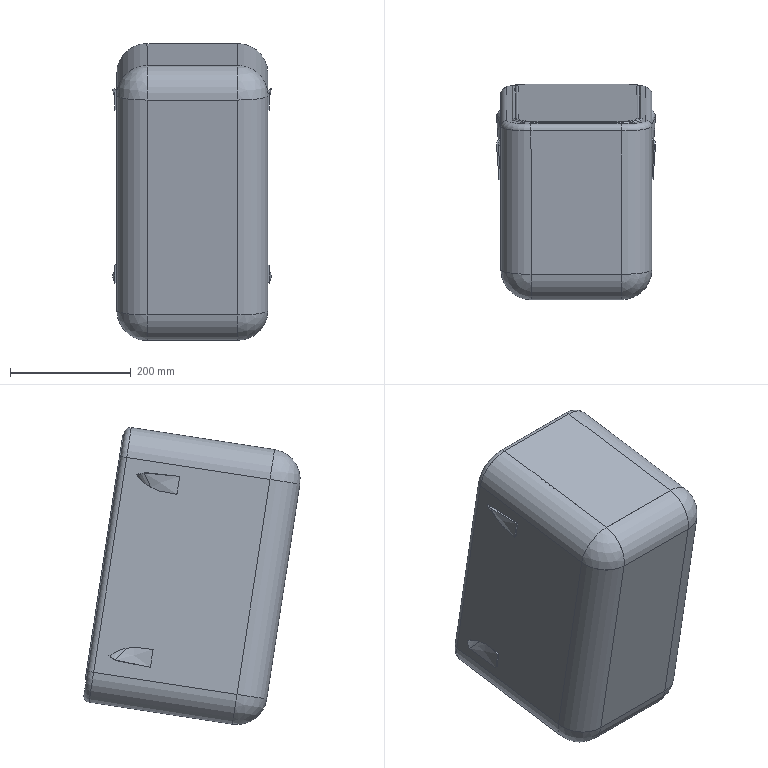Part | SolidWorks | features BaseBody 1 | 1 solid | 155 faces | box 263.41 x 358.039 x 491.823 mm | volume 1227583 mm3 | spline 80 | cylinder 40 | torus 15 | plane 12 | sphere 8 | commonest cylinder face diameters 4 x16 96 x8 100 x8 16 x4 20 x4